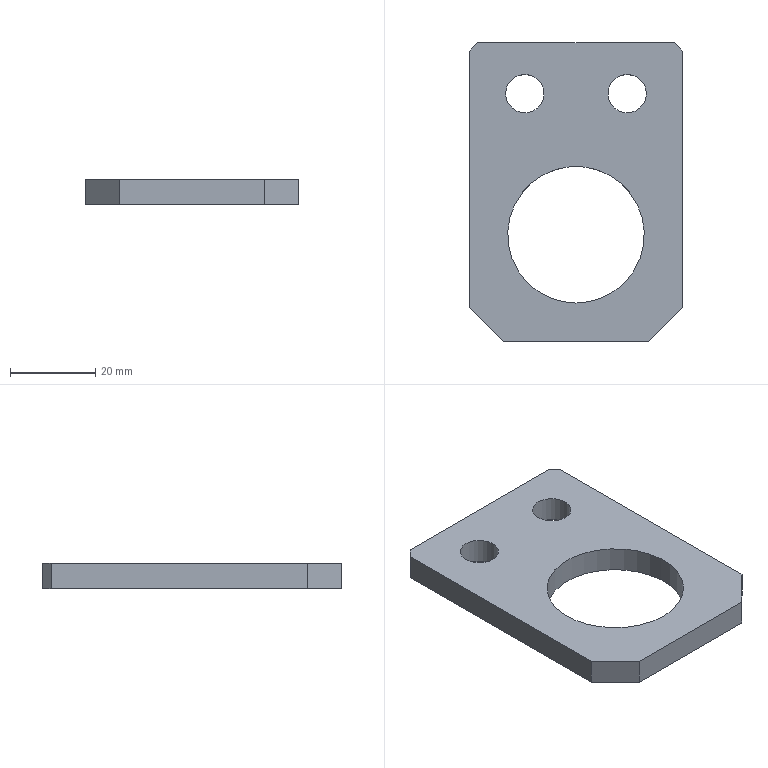Part | NX | features solid 2 | 1 solid | 13 faces | box 50 x 70.05 x 6 mm | volume 15018 mm3 | plane 10 | cylinder 3 | commonest cylinder face diameters 9 x2 32 x1
STEP:
#1=CARTESIAN_POINT('',(-1069.788,-160.721,65.));
#2=VERTEX_POINT('',#1);
#3=CARTESIAN_POINT('',(-1069.788,-100.671,65.));
#4=VERTEX_POINT('',#3);
#5=CARTESIAN_POINT('',(-1069.788,-122.671,65.));
#6=DIRECTION('',(0.,1.,0.));
#7=VECTOR('',#6,1000.);
#8=LINE('',#5,#7);
#9=EDGE_CURVE('',#2,#4,#8,.T.);
#10=ORIENTED_EDGE('',*,*,#9,.T.);
#11=CARTESIAN_POINT('',(-1071.788,-98.671,65.));
#12=VERTEX_POINT('',#11);
#13=CARTESIAN_POINT('',(-1060.788,-109.671,65.));
#14=DIRECTION('',(-0.7071,0.7071,0.));
#15=VECTOR('',#14,1000.);
#16=LINE('',#13,#15);
#17=EDGE_CURVE('',#12,#4,#16,.F.);
#18=ORIENTED_EDGE('',*,*,#17,.F.);
#19=CARTESIAN_POINT('',(-1117.788,-98.671,65.));
#20=VERTEX_POINT('',#19);
#21=CARTESIAN_POINT('',(-1094.788,-98.671,65.));
#22=DIRECTION('',(-1.,0.,0.));
#23=VECTOR('',#22,1000.);
#24=LINE('',#21,#23);
#25=EDGE_CURVE('',#12,#20,#24,.T.);
#26=ORIENTED_EDGE('',*,*,#25,.T.);
#27=CARTESIAN_POINT('',(-1119.788,-100.671,65.));
#28=VERTEX_POINT('',#27);
#29=CARTESIAN_POINT('',(-1128.788,-109.671,65.));
#30=DIRECTION('',(-0.7071,-0.7071,0.));
#31=VECTOR('',#30,1000.);
#32=LINE('',#29,#31);
#33=EDGE_CURVE('',#28,#20,#32,.F.);
#34=ORIENTED_EDGE('',*,*,#33,.F.);
#35=CARTESIAN_POINT('',(-1119.788,-160.721,65.));
#36=VERTEX_POINT('',#35);
#37=CARTESIAN_POINT('',(-1119.788,-122.671,65.));
#38=DIRECTION('',(0.,-1.,0.));
#39=VECTOR('',#38,1000.);
#40=LINE('',#37,#39);
#41=EDGE_CURVE('',#28,#36,#40,.T.);
#42=ORIENTED_EDGE('',*,*,#41,.T.);
#43=CARTESIAN_POINT('',(-1111.788,-168.721,65.));
#44=VERTEX_POINT('',#43);
#45=CARTESIAN_POINT('',(-1125.788,-154.721,65.));
#46=DIRECTION('',(0.7071,-0.7071,0.));
#47=VECTOR('',#46,1000.);
#48=LINE('',#45,#47);
#49=EDGE_CURVE('',#44,#36,#48,.F.);
#50=ORIENTED_EDGE('',*,*,#49,.F.);
#51=CARTESIAN_POINT('',(-1077.788,-168.721,65.));
#52=VERTEX_POINT('',#51);
#53=CARTESIAN_POINT('',(-1094.788,-168.721,65.));
#54=DIRECTION('',(1.,0.,0.));
#55=VECTOR('',#54,1000.);
#56=LINE('',#53,#55);
#57=EDGE_CURVE('',#44,#52,#56,.T.);
#58=ORIENTED_EDGE('',*,*,#57,.T.);
#59=CARTESIAN_POINT('',(-1063.788,-154.721,65.));
#60=DIRECTION('',(0.7071,0.7071,0.));
#61=VECTOR('',#60,1000.);
#62=LINE('',#59,#61);
#63=EDGE_CURVE('',#2,#52,#62,.F.);
#64=ORIENTED_EDGE('',*,*,#63,.F.);
#65=EDGE_LOOP('',(#10,#18,#26,#34,#42,#50,#58,#64));
#66=FACE_BOUND('',#65,.T.);
#67=CARTESIAN_POINT('',(-1106.788,-115.171,65.));
#68=VERTEX_POINT('',#67);
#69=CARTESIAN_POINT('',(-1106.788,-110.671,65.));
#70=DIRECTION('',(0.,0.,1.));
#71=DIRECTION('',(0.,-1.,0.));
#72=AXIS2_PLACEMENT_3D('',#69,#70,#71);
#73=CIRCLE('',#72,4.5);
#74=EDGE_CURVE('',#68,#68,#73,.T.);
#75=ORIENTED_EDGE('',*,*,#74,.F.);
#76=EDGE_LOOP('',(#75));
#77=FACE_BOUND('',#76,.T.);
#78=CARTESIAN_POINT('',(-1082.788,-115.171,65.));
#79=VERTEX_POINT('',#78);
#80=CARTESIAN_POINT('',(-1082.788,-110.671,65.));
#81=DIRECTION('',(0.,0.,1.));
#82=DIRECTION('',(0.,-1.,0.));
#83=AXIS2_PLACEMENT_3D('',#80,#81,#82);
#84=CIRCLE('',#83,4.5);
#85=EDGE_CURVE('',#79,#79,#84,.T.);
#86=ORIENTED_EDGE('',*,*,#85,.F.);
#87=EDGE_LOOP('',(#86));
#88=FACE_BOUND('',#87,.T.);
#89=CARTESIAN_POINT('',(-1094.788,-159.721,65.));
#90=VERTEX_POINT('',#89);
#91=CARTESIAN_POINT('',(-1094.788,-143.721,65.));
#92=DIRECTION('',(0.,0.,1.));
#93=DIRECTION('',(0.,-1.,0.));
#94=AXIS2_PLACEMENT_3D('',#91,#92,#93);
#95=CIRCLE('',#94,16.);
#96=EDGE_CURVE('',#90,#90,#95,.T.);
#97=ORIENTED_EDGE('',*,*,#96,.F.);
#98=EDGE_LOOP('',(#97));
#99=FACE_BOUND('',#98,.T.);
#100=CARTESIAN_POINT('',(-1094.788,-122.671,65.));
#101=DIRECTION('',(0.,0.,1.));
#102=DIRECTION('',(0.,1.,0.));
#103=AXIS2_PLACEMENT_3D('',#100,#101,#102);
#104=PLANE('',#103);
#105=ADVANCED_FACE('',(#66,#77,#88,#99),#104,.T.);
#106=ORIENTED_EDGE('',*,*,#41,.F.);
#107=CARTESIAN_POINT('',(-1119.788,-100.671,59.));
#108=VERTEX_POINT('',#107);
#109=CARTESIAN_POINT('',(-1119.788,-100.671,59.));
#110=DIRECTION('',(0.,0.,1.));
#111=VECTOR('',#110,1000.);
#112=LINE('',#109,#111);
#113=EDGE_CURVE('',#108,#28,#112,.T.);
#114=ORIENTED_EDGE('',*,*,#113,.F.);
#115=CARTESIAN_POINT('',(-1119.788,-160.721,59.));
#116=VERTEX_POINT('',#115);
#117=CARTESIAN_POINT('',(-1119.788,-122.671,59.));
#118=DIRECTION('',(0.,1.,0.));
#119=VECTOR('',#118,1000.);
#120=LINE('',#117,#119);
#121=EDGE_CURVE('',#116,#108,#120,.T.);
#122=ORIENTED_EDGE('',*,*,#121,.F.);
#123=CARTESIAN_POINT('',(-1119.788,-160.721,59.));
#124=DIRECTION('',(0.,0.,-1.));
#125=VECTOR('',#124,1000.);
#126=LINE('',#123,#125);
#127=EDGE_CURVE('',#36,#116,#126,.T.);
#128=ORIENTED_EDGE('',*,*,#127,.F.);
#129=EDGE_LOOP('',(#106,#114,#122,#128));
#130=FACE_BOUND('',#129,.T.);
#131=CARTESIAN_POINT('',(-1119.788,-122.671,59.));
#132=DIRECTION('',(-1.,0.,0.));
#133=DIRECTION('',(0.,0.,-1.));
#134=AXIS2_PLACEMENT_3D('',#131,#132,#133);
#135=PLANE('',#134);
#136=ADVANCED_FACE('',(#130),#135,.T.);
#137=CARTESIAN_POINT('',(-1069.788,-100.671,59.));
#138=VERTEX_POINT('',#137);
#139=CARTESIAN_POINT('',(-1069.788,-160.721,59.));
#140=VERTEX_POINT('',#139);
#141=CARTESIAN_POINT('',(-1069.788,-122.671,59.));
#142=DIRECTION('',(0.,-1.,0.));
#143=VECTOR('',#142,1000.);
#144=LINE('',#141,#143);
#145=EDGE_CURVE('',#138,#140,#144,.T.);
#146=ORIENTED_EDGE('',*,*,#145,.F.);
#147=CARTESIAN_POINT('',(-1069.788,-100.671,59.));
#148=DIRECTION('',(0.,0.,-1.));
#149=VECTOR('',#148,1000.);
#150=LINE('',#147,#149);
#151=EDGE_CURVE('',#4,#138,#150,.T.);
#152=ORIENTED_EDGE('',*,*,#151,.F.);
#153=ORIENTED_EDGE('',*,*,#9,.F.);
#154=CARTESIAN_POINT('',(-1069.788,-160.721,59.));
#155=DIRECTION('',(0.,0.,1.));
#156=VECTOR('',#155,1000.);
#157=LINE('',#154,#156);
#158=EDGE_CURVE('',#140,#2,#157,.T.);
#159=ORIENTED_EDGE('',*,*,#158,.F.);
#160=EDGE_LOOP('',(#146,#152,#153,#159));
#161=FACE_BOUND('',#160,.T.);
#162=CARTESIAN_POINT('',(-1069.788,-122.671,59.));
#163=DIRECTION('',(1.,0.,0.));
#164=DIRECTION('',(0.,0.,1.));
#165=AXIS2_PLACEMENT_3D('',#162,#163,#164);
#166=PLANE('',#165);
#167=ADVANCED_FACE('',(#161),#166,.T.);
#168=ORIENTED_EDGE('',*,*,#121,.T.);
#169=CARTESIAN_POINT('',(-1117.788,-98.671,59.));
#170=VERTEX_POINT('',#169);
#171=CARTESIAN_POINT('',(-1128.788,-109.671,59.));
#172=DIRECTION('',(0.7071,0.7071,0.));
#173=VECTOR('',#172,1000.);
#174=LINE('',#171,#173);
#175=EDGE_CURVE('',#170,#108,#174,.F.);
#176=ORIENTED_EDGE('',*,*,#175,.F.);
#177=CARTESIAN_POINT('',(-1071.788,-98.671,59.));
#178=VERTEX_POINT('',#177);
#179=CARTESIAN_POINT('',(-1094.788,-98.671,59.));
#180=DIRECTION('',(1.,0.,0.));
#181=VECTOR('',#180,1000.);
#182=LINE('',#179,#181);
#183=EDGE_CURVE('',#170,#178,#182,.T.);
#184=ORIENTED_EDGE('',*,*,#183,.T.);
#185=CARTESIAN_POINT('',(-1060.788,-109.671,59.));
#186=DIRECTION('',(0.7071,-0.7071,0.));
#187=VECTOR('',#186,1000.);
#188=LINE('',#185,#187);
#189=EDGE_CURVE('',#138,#178,#188,.F.);
#190=ORIENTED_EDGE('',*,*,#189,.F.);
#191=ORIENTED_EDGE('',*,*,#145,.T.);
#192=CARTESIAN_POINT('',(-1077.788,-168.721,59.));
#193=VERTEX_POINT('',#192);
#194=CARTESIAN_POINT('',(-1063.788,-154.721,59.));
#195=DIRECTION('',(-0.7071,-0.7071,0.));
#196=VECTOR('',#195,1000.);
#197=LINE('',#194,#196);
#198=EDGE_CURVE('',#193,#140,#197,.F.);
#199=ORIENTED_EDGE('',*,*,#198,.F.);
#200=CARTESIAN_POINT('',(-1111.788,-168.721,59.));
#201=VERTEX_POINT('',#200);
#202=CARTESIAN_POINT('',(-1094.788,-168.721,59.));
#203=DIRECTION('',(-1.,0.,0.));
#204=VECTOR('',#203,1000.);
#205=LINE('',#202,#204);
#206=EDGE_CURVE('',#193,#201,#205,.T.);
#207=ORIENTED_EDGE('',*,*,#206,.T.);
#208=CARTESIAN_POINT('',(-1125.788,-154.721,59.));
#209=DIRECTION('',(-0.7071,0.7071,0.));
#210=VECTOR('',#209,1000.);
#211=LINE('',#208,#210);
#212=EDGE_CURVE('',#116,#201,#211,.F.);
#213=ORIENTED_EDGE('',*,*,#212,.F.);
#214=EDGE_LOOP('',(#168,#176,#184,#190,#191,#199,#207,#213));
#215=FACE_BOUND('',#214,.T.);
#216=CARTESIAN_POINT('',(-1106.788,-115.171,59.));
#217=VERTEX_POINT('',#216);
#218=CARTESIAN_POINT('',(-1106.788,-110.671,59.));
#219=DIRECTION('',(0.,0.,1.));
#220=DIRECTION('',(0.,-1.,0.));
#221=AXIS2_PLACEMENT_3D('',#218,#219,#220);
#222=CIRCLE('',#221,4.5);
#223=EDGE_CURVE('',#217,#217,#222,.T.);
#224=ORIENTED_EDGE('',*,*,#223,.T.);
#225=EDGE_LOOP('',(#224));
#226=FACE_BOUND('',#225,.T.);
#227=CARTESIAN_POINT('',(-1082.788,-115.171,59.));
#228=VERTEX_POINT('',#227);
#229=CARTESIAN_POINT('',(-1082.788,-110.671,59.));
#230=DIRECTION('',(0.,0.,1.));
#231=DIRECTION('',(0.,-1.,0.));
#232=AXIS2_PLACEMENT_3D('',#229,#230,#231);
#233=CIRCLE('',#232,4.5);
#234=EDGE_CURVE('',#228,#228,#233,.T.);
#235=ORIENTED_EDGE('',*,*,#234,.T.);
#236=EDGE_LOOP('',(#235));
#237=FACE_BOUND('',#236,.T.);
#238=CARTESIAN_POINT('',(-1094.788,-159.721,59.));
#239=VERTEX_POINT('',#238);
#240=CARTESIAN_POINT('',(-1094.788,-143.721,59.));
#241=DIRECTION('',(0.,0.,1.));
#242=DIRECTION('',(0.,-1.,0.));
#243=AXIS2_PLACEMENT_3D('',#240,#241,#242);
#244=CIRCLE('',#243,16.);
#245=EDGE_CURVE('',#239,#239,#244,.T.);
#246=ORIENTED_EDGE('',*,*,#245,.T.);
#247=EDGE_LOOP('',(#246));
#248=FACE_BOUND('',#247,.T.);
#249=CARTESIAN_POINT('',(-1094.788,-122.671,59.));
#250=DIRECTION('',(0.,0.,-1.));
#251=DIRECTION('',(0.,-1.,0.));
#252=AXIS2_PLACEMENT_3D('',#249,#250,#251);
#253=PLANE('',#252);
#254=ADVANCED_FACE('',(#215,#226,#237,#248),#253,.T.);
#255=ORIENTED_EDGE('',*,*,#183,.F.);
#256=CARTESIAN_POINT('',(-1117.788,-98.671,59.));
#257=DIRECTION('',(0.,0.,-1.));
#258=VECTOR('',#257,1000.);
#259=LINE('',#256,#258);
#260=EDGE_CURVE('',#20,#170,#259,.T.);
#261=ORIENTED_EDGE('',*,*,#260,.F.);
#262=ORIENTED_EDGE('',*,*,#25,.F.);
#263=CARTESIAN_POINT('',(-1071.788,-98.671,59.));
#264=DIRECTION('',(0.,0.,1.));
#265=VECTOR('',#264,1000.);
#266=LINE('',#263,#265);
#267=EDGE_CURVE('',#178,#12,#266,.T.);
#268=ORIENTED_EDGE('',*,*,#267,.F.);
#269=EDGE_LOOP('',(#255,#261,#262,#268));
#270=FACE_BOUND('',#269,.T.);
#271=CARTESIAN_POINT('',(-1094.788,-98.671,59.));
#272=DIRECTION('',(0.,1.,0.));
#273=DIRECTION('',(0.,0.,-1.));
#274=AXIS2_PLACEMENT_3D('',#271,#272,#273);
#275=PLANE('',#274);
#276=ADVANCED_FACE('',(#270),#275,.T.);
#277=ORIENTED_EDGE('',*,*,#189,.T.);
#278=ORIENTED_EDGE('',*,*,#267,.T.);
#279=ORIENTED_EDGE('',*,*,#17,.T.);
#280=ORIENTED_EDGE('',*,*,#151,.T.);
#281=EDGE_LOOP('',(#277,#278,#279,#280));
#282=FACE_BOUND('',#281,.T.);
#283=CARTESIAN_POINT('',(-1071.788,-98.671,59.));
#284=DIRECTION('',(-0.7071,-0.7071,0.));
#285=DIRECTION('',(-0.7071,0.7071,0.));
#286=AXIS2_PLACEMENT_3D('',#283,#284,#285);
#287=PLANE('',#286);
#288=ADVANCED_FACE('',(#282),#287,.F.);
#289=ORIENTED_EDGE('',*,*,#175,.T.);
#290=ORIENTED_EDGE('',*,*,#113,.T.);
#291=ORIENTED_EDGE('',*,*,#33,.T.);
#292=ORIENTED_EDGE('',*,*,#260,.T.);
#293=EDGE_LOOP('',(#289,#290,#291,#292));
#294=FACE_BOUND('',#293,.T.);
#295=CARTESIAN_POINT('',(-1119.788,-100.671,59.));
#296=DIRECTION('',(0.7071,-0.7071,0.));
#297=DIRECTION('',(-0.7071,-0.7071,0.));
#298=AXIS2_PLACEMENT_3D('',#295,#296,#297);
#299=PLANE('',#298);
#300=ADVANCED_FACE('',(#294),#299,.F.);
#301=ORIENTED_EDGE('',*,*,#234,.F.);
#302=EDGE_LOOP('',(#301));
#303=FACE_BOUND('',#302,.T.);
#304=ORIENTED_EDGE('',*,*,#85,.T.);
#305=EDGE_LOOP('',(#304));
#306=FACE_BOUND('',#305,.T.);
#307=CARTESIAN_POINT('',(-1082.788,-110.671,65.));
#308=DIRECTION('',(0.,0.,-1.));
#309=DIRECTION('',(0.,-1.,0.));
#310=AXIS2_PLACEMENT_3D('',#307,#308,#309);
#311=CYLINDRICAL_SURFACE('',#310,4.5);
#312=ADVANCED_FACE('',(#303,#306),#311,.F.);
#313=ORIENTED_EDGE('',*,*,#223,.F.);
#314=EDGE_LOOP('',(#313));
#315=FACE_BOUND('',#314,.T.);
#316=ORIENTED_EDGE('',*,*,#74,.T.);
#317=EDGE_LOOP('',(#316));
#318=FACE_BOUND('',#317,.T.);
#319=CARTESIAN_POINT('',(-1106.788,-110.671,65.));
#320=DIRECTION('',(0.,0.,-1.));
#321=DIRECTION('',(0.,-1.,0.));
#322=AXIS2_PLACEMENT_3D('',#319,#320,#321);
#323=CYLINDRICAL_SURFACE('',#322,4.5);
#324=ADVANCED_FACE('',(#315,#318),#323,.F.);
#325=ORIENTED_EDGE('',*,*,#198,.T.);
#326=ORIENTED_EDGE('',*,*,#158,.T.);
#327=ORIENTED_EDGE('',*,*,#63,.T.);
#328=CARTESIAN_POINT('',(-1077.788,-168.721,59.));
#329=DIRECTION('',(0.,0.,-1.));
#330=VECTOR('',#329,1000.);
#331=LINE('',#328,#330);
#332=EDGE_CURVE('',#52,#193,#331,.T.);
#333=ORIENTED_EDGE('',*,*,#332,.T.);
#334=EDGE_LOOP('',(#325,#326,#327,#333));
#335=FACE_BOUND('',#334,.T.);
#336=CARTESIAN_POINT('',(-1069.788,-160.721,59.));
#337=DIRECTION('',(-0.7071,0.7071,0.));
#338=DIRECTION('',(0.7071,0.7071,0.));
#339=AXIS2_PLACEMENT_3D('',#336,#337,#338);
#340=PLANE('',#339);
#341=ADVANCED_FACE('',(#335),#340,.F.);
#342=ORIENTED_EDGE('',*,*,#57,.F.);
#343=CARTESIAN_POINT('',(-1111.788,-168.721,59.));
#344=DIRECTION('',(0.,0.,1.));
#345=VECTOR('',#344,1000.);
#346=LINE('',#343,#345);
#347=EDGE_CURVE('',#201,#44,#346,.T.);
#348=ORIENTED_EDGE('',*,*,#347,.F.);
#349=ORIENTED_EDGE('',*,*,#206,.F.);
#350=ORIENTED_EDGE('',*,*,#332,.F.);
#351=EDGE_LOOP('',(#342,#348,#349,#350));
#352=FACE_BOUND('',#351,.T.);
#353=CARTESIAN_POINT('',(-1094.788,-168.721,59.));
#354=DIRECTION('',(0.,-1.,0.));
#355=DIRECTION('',(0.,0.,1.));
#356=AXIS2_PLACEMENT_3D('',#353,#354,#355);
#357=PLANE('',#356);
#358=ADVANCED_FACE('',(#352),#357,.T.);
#359=ORIENTED_EDGE('',*,*,#212,.T.);
#360=ORIENTED_EDGE('',*,*,#347,.T.);
#361=ORIENTED_EDGE('',*,*,#49,.T.);
#362=ORIENTED_EDGE('',*,*,#127,.T.);
#363=EDGE_LOOP('',(#359,#360,#361,#362));
#364=FACE_BOUND('',#363,.T.);
#365=CARTESIAN_POINT('',(-1111.788,-168.721,59.));
#366=DIRECTION('',(0.7071,0.7071,0.));
#367=DIRECTION('',(0.7071,-0.7071,0.));
#368=AXIS2_PLACEMENT_3D('',#365,#366,#367);
#369=PLANE('',#368);
#370=ADVANCED_FACE('',(#364),#369,.F.);
#371=ORIENTED_EDGE('',*,*,#245,.F.);
#372=EDGE_LOOP('',(#371));
#373=FACE_BOUND('',#372,.T.);
#374=ORIENTED_EDGE('',*,*,#96,.T.);
#375=EDGE_LOOP('',(#374));
#376=FACE_BOUND('',#375,.T.);
#377=CARTESIAN_POINT('',(-1094.788,-143.721,65.));
#378=DIRECTION('',(0.,0.,-1.));
#379=DIRECTION('',(0.,-1.,0.));
#380=AXIS2_PLACEMENT_3D('',#377,#378,#379);
#381=CYLINDRICAL_SURFACE('',#380,16.);
#382=ADVANCED_FACE('',(#373,#376),#381,.F.);
#383=CLOSED_SHELL('',(#105,#136,#167,#254,#276,#288,#300,#312,#324,#341,#358,#370,#382));
#384=MANIFOLD_SOLID_BREP('',#383);
#385=(LENGTH_UNIT()NAMED_UNIT(*)SI_UNIT(.MILLI.,.METRE.));
#386=UNCERTAINTY_MEASURE_WITH_UNIT(LENGTH_MEASURE(0.00001),#385,'','');
#387=(NAMED_UNIT(*)PLANE_ANGLE_UNIT()SI_UNIT($,.RADIAN.));
#388=(NAMED_UNIT(*)SI_UNIT($,.STERADIAN.)SOLID_ANGLE_UNIT());
#389=(GEOMETRIC_REPRESENTATION_CONTEXT(3)GLOBAL_UNCERTAINTY_ASSIGNED_CONTEXT((#386))GLOBAL_UNIT_ASSIGNED_CONTEXT((#385,#387,#388))REPRESENTATION_CONTEXT('',''));
#390=ADVANCED_BREP_SHAPE_REPRESENTATION('',(#384),#389);